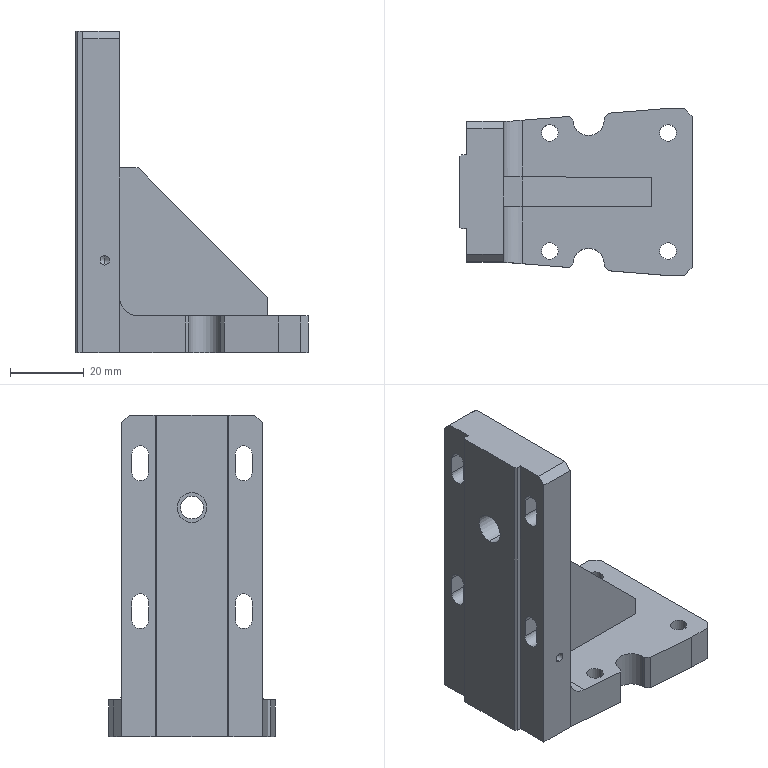Part | SolidWorks | features ICE 10, Chamfer 3, HoleWzd 2, Cut 1, Extrusion 1, Fillet 1, LPattern 1, MirrorPattern 1 | 1 solid | 95 faces | box 62.8 x 45 x 87 mm | volume 61473 mm3 | plane 50 | cylinder 37 | cone 8 | commonest cylinder face diameters 4.5 x16 6 x5 2.5 x4 3.3 x4 6.2 x2 8.1 x2